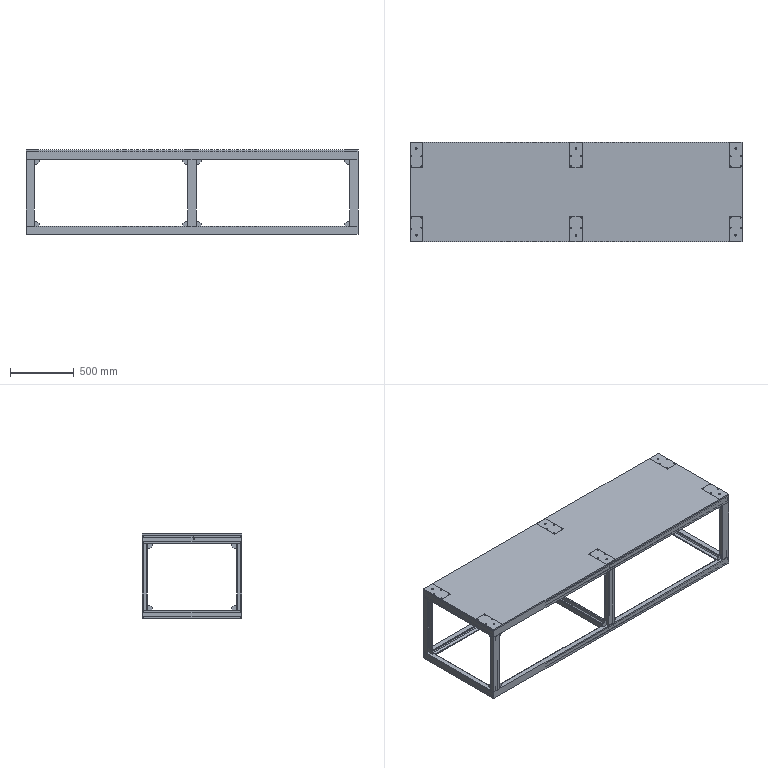Part | STEP file | Box 1_default<machined> | 43 solids | 538 faces | box 2600 x 780 x 662 mm | volume 45698712 mm3 | plane 388 | cylinder 142 | cone 8 | commonest cylinder face diameters 8.5 x56 8 x36 16 x36 12 x14